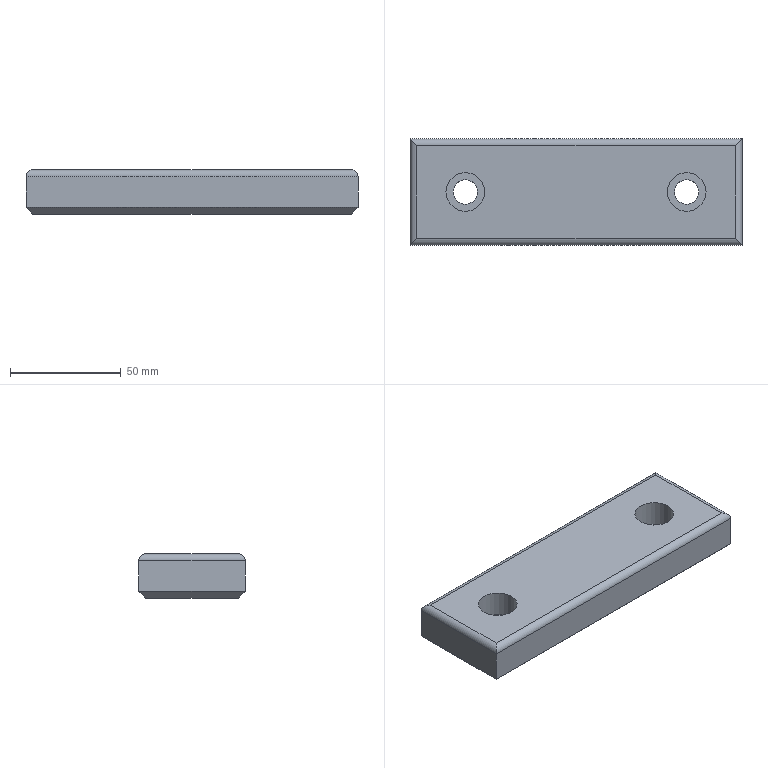Part | NX | features MAIN_BODY 2 | 1 solid | 20 faces | box 150 x 48 x 20 mm | volume 134206 mm3 | plane 12 | cylinder 8 | commonest cylinder face diameters 6 x4 11 x2 17.5 x2
STEP:
#1=CARTESIAN_POINT('',(-245.,291.,-377.));
#2=VERTEX_POINT('',#1);
#3=CARTESIAN_POINT('',(-245.,291.,-363.));
#4=VERTEX_POINT('',#3);
#5=CARTESIAN_POINT('',(-245.,291.,-380.));
#6=DIRECTION('',(0.,0.,1.));
#7=VECTOR('',#6,1000.);
#8=LINE('',#5,#7);
#9=EDGE_CURVE('',#2,#4,#8,.T.);
#10=ORIENTED_EDGE('',*,*,#9,.T.);
#11=CARTESIAN_POINT('',(-245.,339.,-363.));
#12=VERTEX_POINT('',#11);
#13=CARTESIAN_POINT('',(-245.,339.,-363.));
#14=DIRECTION('',(0.,-1.,0.));
#15=VECTOR('',#14,1000.);
#16=LINE('',#13,#15);
#17=EDGE_CURVE('',#12,#4,#16,.T.);
#18=ORIENTED_EDGE('',*,*,#17,.F.);
#19=CARTESIAN_POINT('',(-245.,339.,-377.));
#20=VERTEX_POINT('',#19);
#21=CARTESIAN_POINT('',(-245.,339.,-380.));
#22=DIRECTION('',(0.,0.,1.));
#23=VECTOR('',#22,1000.);
#24=LINE('',#21,#23);
#25=EDGE_CURVE('',#20,#12,#24,.T.);
#26=ORIENTED_EDGE('',*,*,#25,.F.);
#27=CARTESIAN_POINT('',(-245.,339.,-377.));
#28=DIRECTION('',(0.,1.,0.));
#29=VECTOR('',#28,1000.);
#30=LINE('',#27,#29);
#31=EDGE_CURVE('',#2,#20,#30,.T.);
#32=ORIENTED_EDGE('',*,*,#31,.F.);
#33=EDGE_LOOP('',(#10,#18,#26,#32));
#34=FACE_BOUND('',#33,.T.);
#35=CARTESIAN_POINT('',(-245.,339.,-380.));
#36=DIRECTION('',(1.,0.,0.));
#37=DIRECTION('',(0.,0.,1.));
#38=AXIS2_PLACEMENT_3D('',#35,#36,#37);
#39=PLANE('',#38);
#40=ADVANCED_FACE('',(#34),#39,.F.);
#41=CARTESIAN_POINT('',(-95.,291.,-377.));
#42=VERTEX_POINT('',#41);
#43=CARTESIAN_POINT('',(-95.,291.,-363.));
#44=VERTEX_POINT('',#43);
#45=CARTESIAN_POINT('',(-95.,291.,-380.));
#46=DIRECTION('',(0.,0.,1.));
#47=VECTOR('',#46,1000.);
#48=LINE('',#45,#47);
#49=EDGE_CURVE('',#42,#44,#48,.T.);
#50=ORIENTED_EDGE('',*,*,#49,.T.);
#51=CARTESIAN_POINT('',(-245.,291.,-363.));
#52=DIRECTION('',(1.,0.,0.));
#53=VECTOR('',#52,1000.);
#54=LINE('',#51,#53);
#55=EDGE_CURVE('',#4,#44,#54,.T.);
#56=ORIENTED_EDGE('',*,*,#55,.F.);
#57=ORIENTED_EDGE('',*,*,#9,.F.);
#58=CARTESIAN_POINT('',(-245.,291.,-377.));
#59=DIRECTION('',(-1.,0.,0.));
#60=VECTOR('',#59,1000.);
#61=LINE('',#58,#60);
#62=EDGE_CURVE('',#42,#2,#61,.T.);
#63=ORIENTED_EDGE('',*,*,#62,.F.);
#64=EDGE_LOOP('',(#50,#56,#57,#63));
#65=FACE_BOUND('',#64,.T.);
#66=CARTESIAN_POINT('',(-245.,291.,-380.));
#67=DIRECTION('',(0.,1.,0.));
#68=DIRECTION('',(-1.,0.,0.));
#69=AXIS2_PLACEMENT_3D('',#66,#67,#68);
#70=PLANE('',#69);
#71=ADVANCED_FACE('',(#65),#70,.F.);
#72=CARTESIAN_POINT('',(-95.,339.,-377.));
#73=VERTEX_POINT('',#72);
#74=CARTESIAN_POINT('',(-95.,339.,-363.));
#75=VERTEX_POINT('',#74);
#76=CARTESIAN_POINT('',(-95.,339.,-380.));
#77=DIRECTION('',(0.,0.,1.));
#78=VECTOR('',#77,1000.);
#79=LINE('',#76,#78);
#80=EDGE_CURVE('',#73,#75,#79,.T.);
#81=ORIENTED_EDGE('',*,*,#80,.T.);
#82=CARTESIAN_POINT('',(-95.,291.,-363.));
#83=DIRECTION('',(0.,1.,0.));
#84=VECTOR('',#83,1000.);
#85=LINE('',#82,#84);
#86=EDGE_CURVE('',#44,#75,#85,.T.);
#87=ORIENTED_EDGE('',*,*,#86,.F.);
#88=ORIENTED_EDGE('',*,*,#49,.F.);
#89=CARTESIAN_POINT('',(-95.,291.,-377.));
#90=DIRECTION('',(0.,-1.,0.));
#91=VECTOR('',#90,1000.);
#92=LINE('',#89,#91);
#93=EDGE_CURVE('',#73,#42,#92,.T.);
#94=ORIENTED_EDGE('',*,*,#93,.F.);
#95=EDGE_LOOP('',(#81,#87,#88,#94));
#96=FACE_BOUND('',#95,.T.);
#97=CARTESIAN_POINT('',(-95.,291.,-380.));
#98=DIRECTION('',(-1.,0.,0.));
#99=DIRECTION('',(0.,0.,-1.));
#100=AXIS2_PLACEMENT_3D('',#97,#98,#99);
#101=PLANE('',#100);
#102=ADVANCED_FACE('',(#96),#101,.F.);
#103=ORIENTED_EDGE('',*,*,#25,.T.);
#104=CARTESIAN_POINT('',(-95.,339.,-363.));
#105=DIRECTION('',(-1.,0.,0.));
#106=VECTOR('',#105,1000.);
#107=LINE('',#104,#106);
#108=EDGE_CURVE('',#75,#12,#107,.T.);
#109=ORIENTED_EDGE('',*,*,#108,.F.);
#110=ORIENTED_EDGE('',*,*,#80,.F.);
#111=CARTESIAN_POINT('',(-95.,339.,-377.));
#112=DIRECTION('',(1.,0.,0.));
#113=VECTOR('',#112,1000.);
#114=LINE('',#111,#113);
#115=EDGE_CURVE('',#20,#73,#114,.T.);
#116=ORIENTED_EDGE('',*,*,#115,.F.);
#117=EDGE_LOOP('',(#103,#109,#110,#116));
#118=FACE_BOUND('',#117,.T.);
#119=CARTESIAN_POINT('',(-95.,339.,-380.));
#120=DIRECTION('',(0.,-1.,0.));
#121=DIRECTION('',(1.,0.,0.));
#122=AXIS2_PLACEMENT_3D('',#119,#120,#121);
#123=PLANE('',#122);
#124=ADVANCED_FACE('',(#118),#123,.F.);
#125=CARTESIAN_POINT('',(-242.,294.,-380.));
#126=VERTEX_POINT('',#125);
#127=CARTESIAN_POINT('',(-98.,294.,-380.));
#128=VERTEX_POINT('',#127);
#129=CARTESIAN_POINT('',(-95.,294.,-380.));
#130=DIRECTION('',(1.,0.,0.));
#131=VECTOR('',#130,1000.);
#132=LINE('',#129,#131);
#133=EDGE_CURVE('',#126,#128,#132,.T.);
#134=ORIENTED_EDGE('',*,*,#133,.F.);
#135=CARTESIAN_POINT('',(-242.,336.,-380.));
#136=VERTEX_POINT('',#135);
#137=CARTESIAN_POINT('',(-242.,291.,-380.));
#138=DIRECTION('',(0.,-1.,0.));
#139=VECTOR('',#138,1000.);
#140=LINE('',#137,#139);
#141=EDGE_CURVE('',#136,#126,#140,.T.);
#142=ORIENTED_EDGE('',*,*,#141,.F.);
#143=CARTESIAN_POINT('',(-98.,336.,-380.));
#144=VERTEX_POINT('',#143);
#145=CARTESIAN_POINT('',(-245.,336.,-380.));
#146=DIRECTION('',(-1.,0.,0.));
#147=VECTOR('',#146,1000.);
#148=LINE('',#145,#147);
#149=EDGE_CURVE('',#144,#136,#148,.T.);
#150=ORIENTED_EDGE('',*,*,#149,.F.);
#151=CARTESIAN_POINT('',(-98.,339.,-380.));
#152=DIRECTION('',(0.,1.,0.));
#153=VECTOR('',#152,1000.);
#154=LINE('',#151,#153);
#155=EDGE_CURVE('',#128,#144,#154,.T.);
#156=ORIENTED_EDGE('',*,*,#155,.F.);
#157=EDGE_LOOP('',(#134,#142,#150,#156));
#158=FACE_BOUND('',#157,.T.);
#159=CARTESIAN_POINT('',(-114.5,315.,-380.));
#160=VERTEX_POINT('',#159);
#161=CARTESIAN_POINT('',(-120.,315.,-380.));
#162=DIRECTION('',(0.,0.,1.));
#163=DIRECTION('',(1.,0.,0.));
#164=AXIS2_PLACEMENT_3D('',#161,#162,#163);
#165=CIRCLE('',#164,5.5);
#166=EDGE_CURVE('',#160,#160,#165,.T.);
#167=ORIENTED_EDGE('',*,*,#166,.T.);
#168=EDGE_LOOP('',(#167));
#169=FACE_BOUND('',#168,.T.);
#170=CARTESIAN_POINT('',(-214.5,315.,-380.));
#171=VERTEX_POINT('',#170);
#172=CARTESIAN_POINT('',(-220.,315.,-380.));
#173=DIRECTION('',(0.,0.,1.));
#174=DIRECTION('',(1.,0.,0.));
#175=AXIS2_PLACEMENT_3D('',#172,#173,#174);
#176=CIRCLE('',#175,5.5);
#177=EDGE_CURVE('',#171,#171,#176,.T.);
#178=ORIENTED_EDGE('',*,*,#177,.T.);
#179=EDGE_LOOP('',(#178));
#180=FACE_BOUND('',#179,.T.);
#181=CARTESIAN_POINT('',(-245.,291.,-380.));
#182=DIRECTION('',(0.,0.,-1.));
#183=DIRECTION('',(1.,0.,0.));
#184=AXIS2_PLACEMENT_3D('',#181,#182,#183);
#185=PLANE('',#184);
#186=ADVANCED_FACE('',(#158,#169,#180),#185,.T.);
#187=CARTESIAN_POINT('',(-242.,294.,-360.));
#188=VERTEX_POINT('',#187);
#189=CARTESIAN_POINT('',(-242.,336.,-360.));
#190=VERTEX_POINT('',#189);
#191=CARTESIAN_POINT('',(-242.,291.,-360.));
#192=DIRECTION('',(0.,-1.,0.));
#193=VECTOR('',#192,1000.);
#194=LINE('',#191,#193);
#195=EDGE_CURVE('',#188,#190,#194,.F.);
#196=ORIENTED_EDGE('',*,*,#195,.F.);
#197=CARTESIAN_POINT('',(-98.,294.,-360.));
#198=VERTEX_POINT('',#197);
#199=CARTESIAN_POINT('',(-245.,294.,-360.));
#200=DIRECTION('',(1.,0.,0.));
#201=VECTOR('',#200,1000.);
#202=LINE('',#199,#201);
#203=EDGE_CURVE('',#198,#188,#202,.F.);
#204=ORIENTED_EDGE('',*,*,#203,.F.);
#205=CARTESIAN_POINT('',(-98.,336.,-360.));
#206=VERTEX_POINT('',#205);
#207=CARTESIAN_POINT('',(-98.,291.,-360.));
#208=DIRECTION('',(0.,1.,0.));
#209=VECTOR('',#208,1000.);
#210=LINE('',#207,#209);
#211=EDGE_CURVE('',#206,#198,#210,.F.);
#212=ORIENTED_EDGE('',*,*,#211,.F.);
#213=CARTESIAN_POINT('',(-245.,336.,-360.));
#214=DIRECTION('',(-1.,0.,0.));
#215=VECTOR('',#214,1000.);
#216=LINE('',#213,#215);
#217=EDGE_CURVE('',#190,#206,#216,.F.);
#218=ORIENTED_EDGE('',*,*,#217,.F.);
#219=EDGE_LOOP('',(#196,#204,#212,#218));
#220=FACE_BOUND('',#219,.T.);
#221=CARTESIAN_POINT('',(-111.25,315.,-360.));
#222=VERTEX_POINT('',#221);
#223=CARTESIAN_POINT('',(-120.,315.,-360.));
#224=DIRECTION('',(0.,0.,1.));
#225=DIRECTION('',(1.,0.,0.));
#226=AXIS2_PLACEMENT_3D('',#223,#224,#225);
#227=CIRCLE('',#226,8.75);
#228=EDGE_CURVE('',#222,#222,#227,.T.);
#229=ORIENTED_EDGE('',*,*,#228,.F.);
#230=EDGE_LOOP('',(#229));
#231=FACE_BOUND('',#230,.T.);
#232=CARTESIAN_POINT('',(-211.25,315.,-360.));
#233=VERTEX_POINT('',#232);
#234=CARTESIAN_POINT('',(-220.,315.,-360.));
#235=DIRECTION('',(0.,0.,1.));
#236=DIRECTION('',(1.,0.,0.));
#237=AXIS2_PLACEMENT_3D('',#234,#235,#236);
#238=CIRCLE('',#237,8.75);
#239=EDGE_CURVE('',#233,#233,#238,.T.);
#240=ORIENTED_EDGE('',*,*,#239,.F.);
#241=EDGE_LOOP('',(#240));
#242=FACE_BOUND('',#241,.T.);
#243=CARTESIAN_POINT('',(-245.,291.,-360.));
#244=DIRECTION('',(0.,0.,-1.));
#245=DIRECTION('',(1.,0.,0.));
#246=AXIS2_PLACEMENT_3D('',#243,#244,#245);
#247=PLANE('',#246);
#248=ADVANCED_FACE('',(#220,#231,#242),#247,.F.);
#249=ORIENTED_EDGE('',*,*,#177,.F.);
#250=EDGE_LOOP('',(#249));
#251=FACE_BOUND('',#250,.T.);
#252=CARTESIAN_POINT('',(-214.5,315.,-372.));
#253=VERTEX_POINT('',#252);
#254=CARTESIAN_POINT('',(-220.,315.,-372.));
#255=DIRECTION('',(0.,0.,1.));
#256=DIRECTION('',(1.,0.,0.));
#257=AXIS2_PLACEMENT_3D('',#254,#255,#256);
#258=CIRCLE('',#257,5.5);
#259=EDGE_CURVE('',#253,#253,#258,.T.);
#260=ORIENTED_EDGE('',*,*,#259,.T.);
#261=EDGE_LOOP('',(#260));
#262=FACE_BOUND('',#261,.T.);
#263=CARTESIAN_POINT('',(-220.,315.,-410.));
#264=DIRECTION('',(0.,0.,-1.));
#265=DIRECTION('',(1.,0.,0.));
#266=AXIS2_PLACEMENT_3D('',#263,#264,#265);
#267=CYLINDRICAL_SURFACE('',#266,5.5);
#268=ADVANCED_FACE('',(#251,#262),#267,.F.);
#269=ORIENTED_EDGE('',*,*,#259,.F.);
#270=EDGE_LOOP('',(#269));
#271=FACE_BOUND('',#270,.T.);
#272=CARTESIAN_POINT('',(-211.25,315.,-372.));
#273=VERTEX_POINT('',#272);
#274=CARTESIAN_POINT('',(-220.,315.,-372.));
#275=DIRECTION('',(0.,0.,1.));
#276=DIRECTION('',(1.,0.,0.));
#277=AXIS2_PLACEMENT_3D('',#274,#275,#276);
#278=CIRCLE('',#277,8.75);
#279=EDGE_CURVE('',#273,#273,#278,.T.);
#280=ORIENTED_EDGE('',*,*,#279,.T.);
#281=EDGE_LOOP('',(#280));
#282=FACE_BOUND('',#281,.T.);
#283=CARTESIAN_POINT('',(-220.,315.,-372.));
#284=DIRECTION('',(0.,0.,-1.));
#285=DIRECTION('',(1.,0.,0.));
#286=AXIS2_PLACEMENT_3D('',#283,#284,#285);
#287=PLANE('',#286);
#288=ADVANCED_FACE('',(#271,#282),#287,.F.);
#289=ORIENTED_EDGE('',*,*,#279,.F.);
#290=EDGE_LOOP('',(#289));
#291=FACE_BOUND('',#290,.T.);
#292=ORIENTED_EDGE('',*,*,#239,.T.);
#293=EDGE_LOOP('',(#292));
#294=FACE_BOUND('',#293,.T.);
#295=CARTESIAN_POINT('',(-220.,315.,-360.));
#296=DIRECTION('',(0.,0.,-1.));
#297=DIRECTION('',(1.,0.,0.));
#298=AXIS2_PLACEMENT_3D('',#295,#296,#297);
#299=CYLINDRICAL_SURFACE('',#298,8.75);
#300=ADVANCED_FACE('',(#291,#294),#299,.F.);
#301=ORIENTED_EDGE('',*,*,#166,.F.);
#302=EDGE_LOOP('',(#301));
#303=FACE_BOUND('',#302,.T.);
#304=CARTESIAN_POINT('',(-114.5,315.,-372.));
#305=VERTEX_POINT('',#304);
#306=CARTESIAN_POINT('',(-120.,315.,-372.));
#307=DIRECTION('',(0.,0.,1.));
#308=DIRECTION('',(1.,0.,0.));
#309=AXIS2_PLACEMENT_3D('',#306,#307,#308);
#310=CIRCLE('',#309,5.5);
#311=EDGE_CURVE('',#305,#305,#310,.T.);
#312=ORIENTED_EDGE('',*,*,#311,.T.);
#313=EDGE_LOOP('',(#312));
#314=FACE_BOUND('',#313,.T.);
#315=CARTESIAN_POINT('',(-120.,315.,-410.));
#316=DIRECTION('',(0.,0.,-1.));
#317=DIRECTION('',(1.,0.,0.));
#318=AXIS2_PLACEMENT_3D('',#315,#316,#317);
#319=CYLINDRICAL_SURFACE('',#318,5.5);
#320=ADVANCED_FACE('',(#303,#314),#319,.F.);
#321=ORIENTED_EDGE('',*,*,#311,.F.);
#322=EDGE_LOOP('',(#321));
#323=FACE_BOUND('',#322,.T.);
#324=CARTESIAN_POINT('',(-111.25,315.,-372.));
#325=VERTEX_POINT('',#324);
#326=CARTESIAN_POINT('',(-120.,315.,-372.));
#327=DIRECTION('',(0.,0.,1.));
#328=DIRECTION('',(1.,0.,0.));
#329=AXIS2_PLACEMENT_3D('',#326,#327,#328);
#330=CIRCLE('',#329,8.75);
#331=EDGE_CURVE('',#325,#325,#330,.T.);
#332=ORIENTED_EDGE('',*,*,#331,.T.);
#333=EDGE_LOOP('',(#332));
#334=FACE_BOUND('',#333,.T.);
#335=CARTESIAN_POINT('',(-120.,315.,-372.));
#336=DIRECTION('',(0.,0.,-1.));
#337=DIRECTION('',(1.,0.,0.));
#338=AXIS2_PLACEMENT_3D('',#335,#336,#337);
#339=PLANE('',#338);
#340=ADVANCED_FACE('',(#323,#334),#339,.F.);
#341=ORIENTED_EDGE('',*,*,#331,.F.);
#342=EDGE_LOOP('',(#341));
#343=FACE_BOUND('',#342,.T.);
#344=ORIENTED_EDGE('',*,*,#228,.T.);
#345=EDGE_LOOP('',(#344));
#346=FACE_BOUND('',#345,.T.);
#347=CARTESIAN_POINT('',(-120.,315.,-360.));
#348=DIRECTION('',(0.,0.,-1.));
#349=DIRECTION('',(1.,0.,0.));
#350=AXIS2_PLACEMENT_3D('',#347,#348,#349);
#351=CYLINDRICAL_SURFACE('',#350,8.75);
#352=ADVANCED_FACE('',(#343,#346),#351,.F.);
#353=CARTESIAN_POINT('',(-242.,294.,-363.));
#354=DIRECTION('',(-0.7071,0.7071,0.));
#355=DIRECTION('',(-0.7071,-0.7071,0.));
#356=AXIS2_PLACEMENT_3D('',#353,#354,#355);
#357=ELLIPSE('',#356,4.243,3.);
#358=EDGE_CURVE('',#188,#4,#357,.F.);
#359=ORIENTED_EDGE('',*,*,#358,.T.);
#360=ORIENTED_EDGE('',*,*,#55,.T.);
#361=CARTESIAN_POINT('',(-98.,294.,-363.));
#362=DIRECTION('',(-0.7071,-0.7071,0.));
#363=DIRECTION('',(0.7071,-0.7071,0.));
#364=AXIS2_PLACEMENT_3D('',#361,#362,#363);
#365=ELLIPSE('',#364,4.243,3.);
#366=EDGE_CURVE('',#44,#198,#365,.T.);
#367=ORIENTED_EDGE('',*,*,#366,.T.);
#368=ORIENTED_EDGE('',*,*,#203,.T.);
#369=EDGE_LOOP('',(#359,#360,#367,#368));
#370=FACE_BOUND('',#369,.T.);
#371=CARTESIAN_POINT('',(-245.,294.,-363.));
#372=DIRECTION('',(1.,0.,0.));
#373=DIRECTION('',(0.,1.,0.));
#374=AXIS2_PLACEMENT_3D('',#371,#372,#373);
#375=CYLINDRICAL_SURFACE('',#374,3.);
#376=ADVANCED_FACE('',(#370),#375,.T.);
#377=ORIENTED_EDGE('',*,*,#366,.F.);
#378=ORIENTED_EDGE('',*,*,#86,.T.);
#379=CARTESIAN_POINT('',(-98.,336.,-363.));
#380=DIRECTION('',(0.7071,-0.7071,0.));
#381=DIRECTION('',(0.7071,0.7071,0.));
#382=AXIS2_PLACEMENT_3D('',#379,#380,#381);
#383=ELLIPSE('',#382,4.243,3.);
#384=EDGE_CURVE('',#75,#206,#383,.T.);
#385=ORIENTED_EDGE('',*,*,#384,.T.);
#386=ORIENTED_EDGE('',*,*,#211,.T.);
#387=EDGE_LOOP('',(#377,#378,#385,#386));
#388=FACE_BOUND('',#387,.T.);
#389=CARTESIAN_POINT('',(-98.,291.,-363.));
#390=DIRECTION('',(0.,1.,0.));
#391=DIRECTION('',(0.,0.,-1.));
#392=AXIS2_PLACEMENT_3D('',#389,#390,#391);
#393=CYLINDRICAL_SURFACE('',#392,3.);
#394=ADVANCED_FACE('',(#388),#393,.T.);
#395=ORIENTED_EDGE('',*,*,#358,.F.);
#396=ORIENTED_EDGE('',*,*,#195,.T.);
#397=CARTESIAN_POINT('',(-242.,336.,-363.));
#398=DIRECTION('',(0.7071,0.7071,0.));
#399=DIRECTION('',(0.7071,-0.7071,0.));
#400=AXIS2_PLACEMENT_3D('',#397,#398,#399);
#401=ELLIPSE('',#400,4.243,3.);
#402=EDGE_CURVE('',#190,#12,#401,.F.);
#403=ORIENTED_EDGE('',*,*,#402,.T.);
#404=ORIENTED_EDGE('',*,*,#17,.T.);
#405=EDGE_LOOP('',(#395,#396,#403,#404));
#406=FACE_BOUND('',#405,.T.);
#407=CARTESIAN_POINT('',(-242.,339.,-363.));
#408=DIRECTION('',(0.,-1.,0.));
#409=DIRECTION('',(0.,0.,1.));
#410=AXIS2_PLACEMENT_3D('',#407,#408,#409);
#411=CYLINDRICAL_SURFACE('',#410,3.);
#412=ADVANCED_FACE('',(#406),#411,.T.);
#413=ORIENTED_EDGE('',*,*,#384,.F.);
#414=ORIENTED_EDGE('',*,*,#108,.T.);
#415=ORIENTED_EDGE('',*,*,#402,.F.);
#416=ORIENTED_EDGE('',*,*,#217,.T.);
#417=EDGE_LOOP('',(#413,#414,#415,#416));
#418=FACE_BOUND('',#417,.T.);
#419=CARTESIAN_POINT('',(-95.,336.,-363.));
#420=DIRECTION('',(-1.,0.,0.));
#421=DIRECTION('',(0.,-1.,0.));
#422=AXIS2_PLACEMENT_3D('',#419,#420,#421);
#423=CYLINDRICAL_SURFACE('',#422,3.);
#424=ADVANCED_FACE('',(#418),#423,.T.);
#425=CARTESIAN_POINT('',(-243.,337.,-379.));
#426=DIRECTION('',(0.5774,-0.5774,-0.5774));
#427=VECTOR('',#426,1000.);
#428=LINE('',#425,#427);
#429=EDGE_CURVE('',#20,#136,#428,.T.);
#430=ORIENTED_EDGE('',*,*,#429,.T.);
#431=ORIENTED_EDGE('',*,*,#141,.T.);
#432=CARTESIAN_POINT('',(-243.,293.,-379.));
#433=DIRECTION('',(0.5774,0.5774,-0.5774));
#434=VECTOR('',#433,1000.);
#435=LINE('',#432,#434);
#436=EDGE_CURVE('',#126,#2,#435,.F.);
#437=ORIENTED_EDGE('',*,*,#436,.T.);
#438=ORIENTED_EDGE('',*,*,#31,.T.);
#439=EDGE_LOOP('',(#430,#431,#437,#438));
#440=FACE_BOUND('',#439,.T.);
#441=CARTESIAN_POINT('',(-242.,291.,-380.));
#442=DIRECTION('',(-0.7071,0.,-0.7071));
#443=DIRECTION('',(0.7071,0.,-0.7071));
#444=AXIS2_PLACEMENT_3D('',#441,#442,#443);
#445=PLANE('',#444);
#446=ADVANCED_FACE('',(#440),#445,.T.);
#447=ORIENTED_EDGE('',*,*,#436,.F.);
#448=ORIENTED_EDGE('',*,*,#133,.T.);
#449=CARTESIAN_POINT('',(-147.,343.,-429.));
#450=DIRECTION('',(-0.5774,0.5774,-0.5774));
#451=VECTOR('',#450,1000.);
#452=LINE('',#449,#451);
#453=EDGE_CURVE('',#128,#42,#452,.F.);
#454=ORIENTED_EDGE('',*,*,#453,.T.);
#455=ORIENTED_EDGE('',*,*,#62,.T.);
#456=EDGE_LOOP('',(#447,#448,#454,#455));
#457=FACE_BOUND('',#456,.T.);
#458=CARTESIAN_POINT('',(-245.,294.,-380.));
#459=DIRECTION('',(0.,-0.7071,-0.7071));
#460=DIRECTION('',(0.,-0.7071,0.7071));
#461=AXIS2_PLACEMENT_3D('',#458,#459,#460);
#462=PLANE('',#461);
#463=ADVANCED_FACE('',(#457),#462,.T.);
#464=ORIENTED_EDGE('',*,*,#429,.F.);
#465=ORIENTED_EDGE('',*,*,#115,.T.);
#466=CARTESIAN_POINT('',(-147.,287.,-429.));
#467=DIRECTION('',(0.5774,0.5774,0.5774));
#468=VECTOR('',#467,1000.);
#469=LINE('',#466,#468);
#470=EDGE_CURVE('',#73,#144,#469,.F.);
#471=ORIENTED_EDGE('',*,*,#470,.T.);
#472=ORIENTED_EDGE('',*,*,#149,.T.);
#473=EDGE_LOOP('',(#464,#465,#471,#472));
#474=FACE_BOUND('',#473,.T.);
#475=CARTESIAN_POINT('',(-245.,336.,-380.));
#476=DIRECTION('',(0.,0.7071,-0.7071));
#477=DIRECTION('',(0.,-0.7071,-0.7071));
#478=AXIS2_PLACEMENT_3D('',#475,#476,#477);
#479=PLANE('',#478);
#480=ADVANCED_FACE('',(#474),#479,.T.);
#481=ORIENTED_EDGE('',*,*,#453,.F.);
#482=ORIENTED_EDGE('',*,*,#155,.T.);
#483=ORIENTED_EDGE('',*,*,#470,.F.);
#484=ORIENTED_EDGE('',*,*,#93,.T.);
#485=EDGE_LOOP('',(#481,#482,#483,#484));
#486=FACE_BOUND('',#485,.T.);
#487=CARTESIAN_POINT('',(-98.,291.,-380.));
#488=DIRECTION('',(0.7071,0.,-0.7071));
#489=DIRECTION('',(0.7071,0.,0.7071));
#490=AXIS2_PLACEMENT_3D('',#487,#488,#489);
#491=PLANE('',#490);
#492=ADVANCED_FACE('',(#486),#491,.T.);
#493=CLOSED_SHELL('',(#40,#71,#102,#124,#186,#248,#268,#288,#300,#320,#340,#352,#376,#394,#412,#424,#446,#463,#480,#492));
#494=MANIFOLD_SOLID_BREP('',#493);
#495=(LENGTH_UNIT()NAMED_UNIT(*)SI_UNIT(.MILLI.,.METRE.));
#496=UNCERTAINTY_MEASURE_WITH_UNIT(LENGTH_MEASURE(0.00001),#495,'','');
#497=(NAMED_UNIT(*)PLANE_ANGLE_UNIT()SI_UNIT($,.RADIAN.));
#498=(NAMED_UNIT(*)SI_UNIT($,.STERADIAN.)SOLID_ANGLE_UNIT());
#499=(GEOMETRIC_REPRESENTATION_CONTEXT(3)GLOBAL_UNCERTAINTY_ASSIGNED_CONTEXT((#496))GLOBAL_UNIT_ASSIGNED_CONTEXT((#495,#497,#498))REPRESENTATION_CONTEXT('',''));
#500=ADVANCED_BREP_SHAPE_REPRESENTATION('',(#494),#499);